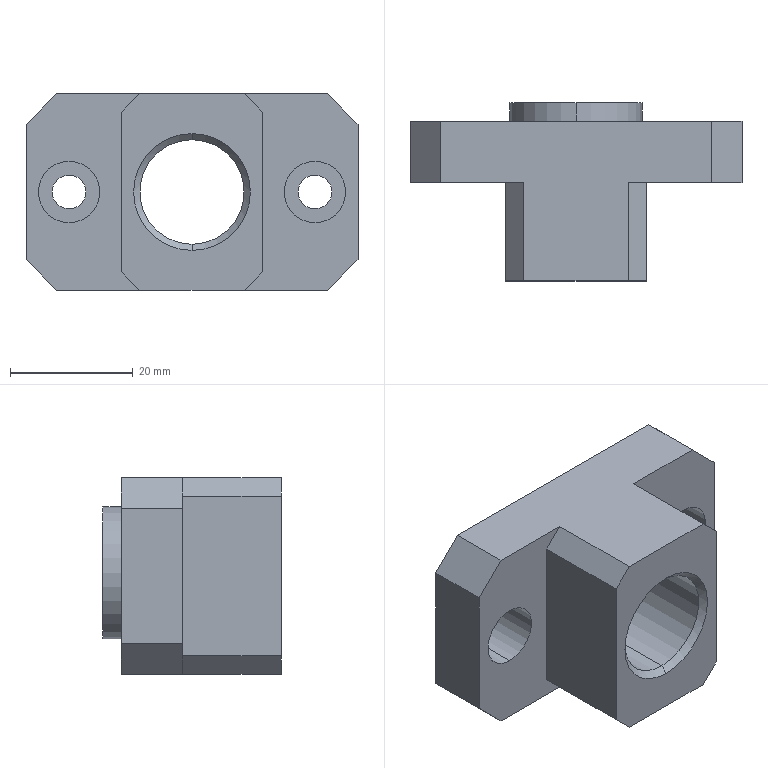Part | SolidWorks | features Chamfer 4, HoleWzd 2, Extrusion 1, ICE 1 | 1 solid | 37 faces | box 54 x 29 x 32 mm | volume 21498 mm3 | plane 21 | cylinder 12 | cone 4 | commonest cylinder face diameters 5.5 x4 10 x4 17 x2 21.5 x2
STEP:
#1=CARTESIAN_POINT('',(0.,-15.009,24.5));
#2=VERTEX_POINT('',#1);
#3=CARTESIAN_POINT('',(0.,-15.009,7.5));
#4=VERTEX_POINT('',#3);
#5=CARTESIAN_POINT('',(0.,-15.009,16.));
#6=DIRECTION('',(0.,-1.,0.));
#7=DIRECTION('',(0.,0.,1.));
#8=AXIS2_PLACEMENT_3D('',#5,#6,#7);
#9=CIRCLE('',#8,8.5);
#10=EDGE_CURVE('',#2,#4,#9,.T.);
#11=ORIENTED_EDGE('',*,*,#10,.F.);
#12=CARTESIAN_POINT('',(0.,-16.009,25.5));
#13=VERTEX_POINT('',#12);
#14=CARTESIAN_POINT('',(0.,-15.009,24.5));
#15=DIRECTION('',(0.,-0.7071,0.7071));
#16=VECTOR('',#15,1000.);
#17=LINE('',#14,#16);
#18=EDGE_CURVE('',#2,#13,#17,.T.);
#19=ORIENTED_EDGE('',*,*,#18,.T.);
#20=CARTESIAN_POINT('',(0.,-16.009,6.5));
#21=VERTEX_POINT('',#20);
#22=CARTESIAN_POINT('',(0.,-16.009,16.));
#23=DIRECTION('',(0.,1.,0.));
#24=DIRECTION('',(0.,0.,1.));
#25=AXIS2_PLACEMENT_3D('',#22,#23,#24);
#26=CIRCLE('',#25,9.5);
#27=EDGE_CURVE('',#21,#13,#26,.T.);
#28=ORIENTED_EDGE('',*,*,#27,.F.);
#29=CARTESIAN_POINT('',(0.,-15.009,7.5));
#30=DIRECTION('',(0.,-0.7071,-0.7071));
#31=VECTOR('',#30,1000.);
#32=LINE('',#29,#31);
#33=EDGE_CURVE('',#4,#21,#32,.T.);
#34=ORIENTED_EDGE('',*,*,#33,.F.);
#35=EDGE_LOOP('',(#11,#19,#28,#34));
#36=FACE_OUTER_BOUND('',#35,.T.);
#37=CARTESIAN_POINT('',(0.,-15.009,16.));
#38=DIRECTION('',(0.,-1.,0.));
#39=DIRECTION('',(0.,0.,-1.));
#40=AXIS2_PLACEMENT_3D('',#37,#38,#39);
#41=CONICAL_SURFACE('',#40,8.5,0.7854);
#42=ADVANCED_FACE('',(#36),#41,.F.);
#43=CARTESIAN_POINT('',(0.,12.491,7.5));
#44=VERTEX_POINT('',#43);
#45=CARTESIAN_POINT('',(0.,12.491,24.5));
#46=VERTEX_POINT('',#45);
#47=CARTESIAN_POINT('',(0.,12.491,16.));
#48=DIRECTION('',(0.,1.,0.));
#49=DIRECTION('',(0.,0.,1.));
#50=AXIS2_PLACEMENT_3D('',#47,#48,#49);
#51=CIRCLE('',#50,8.5);
#52=EDGE_CURVE('',#44,#46,#51,.T.);
#53=ORIENTED_EDGE('',*,*,#52,.F.);
#54=CARTESIAN_POINT('',(0.,12.991,7.));
#55=VERTEX_POINT('',#54);
#56=CARTESIAN_POINT('',(0.,12.991,7.));
#57=DIRECTION('',(0.,0.7071,-0.7071));
#58=VECTOR('',#57,1000.);
#59=LINE('',#56,#58);
#60=EDGE_CURVE('',#44,#55,#59,.T.);
#61=ORIENTED_EDGE('',*,*,#60,.T.);
#62=CARTESIAN_POINT('',(0.,12.991,25.));
#63=VERTEX_POINT('',#62);
#64=CARTESIAN_POINT('',(0.,12.991,16.));
#65=DIRECTION('',(0.,-1.,0.));
#66=DIRECTION('',(0.,0.,1.));
#67=AXIS2_PLACEMENT_3D('',#64,#65,#66);
#68=CIRCLE('',#67,9.);
#69=EDGE_CURVE('',#63,#55,#68,.T.);
#70=ORIENTED_EDGE('',*,*,#69,.F.);
#71=CARTESIAN_POINT('',(0.,12.991,25.));
#72=DIRECTION('',(0.,0.7071,0.7071));
#73=VECTOR('',#72,1000.);
#74=LINE('',#71,#73);
#75=EDGE_CURVE('',#46,#63,#74,.T.);
#76=ORIENTED_EDGE('',*,*,#75,.F.);
#77=EDGE_LOOP('',(#53,#61,#70,#76));
#78=FACE_OUTER_BOUND('',#77,.T.);
#79=CARTESIAN_POINT('',(0.,12.991,16.));
#80=DIRECTION('',(0.,1.,0.));
#81=DIRECTION('',(0.,0.,1.));
#82=AXIS2_PLACEMENT_3D('',#79,#80,#81);
#83=CONICAL_SURFACE('',#82,9.,0.7854);
#84=ADVANCED_FACE('',(#78),#83,.F.);
#85=ORIENTED_EDGE('',*,*,#52,.T.);
#86=CARTESIAN_POINT('',(0.,-16.009,24.5));
#87=DIRECTION('',(0.,-1.,0.));
#88=VECTOR('',#87,1000.);
#89=LINE('',#86,#88);
#90=EDGE_CURVE('',#46,#2,#89,.T.);
#91=ORIENTED_EDGE('',*,*,#90,.T.);
#92=ORIENTED_EDGE('',*,*,#10,.T.);
#93=CARTESIAN_POINT('',(0.,-16.009,7.5));
#94=DIRECTION('',(0.,-1.,0.));
#95=VECTOR('',#94,1000.);
#96=LINE('',#93,#95);
#97=EDGE_CURVE('',#44,#4,#96,.T.);
#98=ORIENTED_EDGE('',*,*,#97,.F.);
#99=EDGE_LOOP('',(#85,#91,#92,#98));
#100=FACE_OUTER_BOUND('',#99,.T.);
#101=CARTESIAN_POINT('',(0.,-16.009,16.));
#102=DIRECTION('',(0.,-1.,0.));
#103=DIRECTION('',(0.,0.,-1.));
#104=AXIS2_PLACEMENT_3D('',#101,#102,#103);
#105=CYLINDRICAL_SURFACE('',#104,8.5);
#106=ADVANCED_FACE('',(#100),#105,.F.);
#107=CARTESIAN_POINT('',(20.,6.991,21.));
#108=VERTEX_POINT('',#107);
#109=CARTESIAN_POINT('',(20.,6.991,11.));
#110=VERTEX_POINT('',#109);
#111=CARTESIAN_POINT('',(20.,6.991,16.));
#112=DIRECTION('',(0.,-1.,0.));
#113=DIRECTION('',(0.,0.,-1.));
#114=AXIS2_PLACEMENT_3D('',#111,#112,#113);
#115=CIRCLE('',#114,5.);
#116=EDGE_CURVE('',#108,#110,#115,.T.);
#117=ORIENTED_EDGE('',*,*,#116,.F.);
#118=CARTESIAN_POINT('',(20.,-0.00863,21.));
#119=VERTEX_POINT('',#118);
#120=CARTESIAN_POINT('',(20.,-0.00863,21.));
#121=DIRECTION('',(0.,-1.,0.));
#122=VECTOR('',#121,1000.);
#123=LINE('',#120,#122);
#124=EDGE_CURVE('',#108,#119,#123,.T.);
#125=ORIENTED_EDGE('',*,*,#124,.T.);
#126=CARTESIAN_POINT('',(20.,-0.00863,11.));
#127=VERTEX_POINT('',#126);
#128=CARTESIAN_POINT('',(20.,-0.00863,16.));
#129=DIRECTION('',(0.,-1.,0.));
#130=DIRECTION('',(0.,0.,-1.));
#131=AXIS2_PLACEMENT_3D('',#128,#129,#130);
#132=CIRCLE('',#131,5.);
#133=EDGE_CURVE('',#119,#127,#132,.T.);
#134=ORIENTED_EDGE('',*,*,#133,.T.);
#135=CARTESIAN_POINT('',(20.,-0.00863,11.));
#136=DIRECTION('',(0.,-1.,0.));
#137=VECTOR('',#136,1000.);
#138=LINE('',#135,#137);
#139=EDGE_CURVE('',#110,#127,#138,.T.);
#140=ORIENTED_EDGE('',*,*,#139,.F.);
#141=EDGE_LOOP('',(#117,#125,#134,#140));
#142=FACE_OUTER_BOUND('',#141,.T.);
#143=CARTESIAN_POINT('',(20.,-0.00863,16.));
#144=DIRECTION('',(0.,-1.,0.));
#145=DIRECTION('',(0.,0.,-1.));
#146=AXIS2_PLACEMENT_3D('',#143,#144,#145);
#147=CYLINDRICAL_SURFACE('',#146,5.);
#148=ADVANCED_FACE('',(#142),#147,.F.);
#149=CARTESIAN_POINT('',(20.,9.991,18.75));
#150=VERTEX_POINT('',#149);
#151=CARTESIAN_POINT('',(20.,9.991,13.25));
#152=VERTEX_POINT('',#151);
#153=CARTESIAN_POINT('',(20.,9.991,16.));
#154=DIRECTION('',(0.,-1.,0.));
#155=DIRECTION('',(0.,0.,-1.));
#156=AXIS2_PLACEMENT_3D('',#153,#154,#155);
#157=CIRCLE('',#156,2.75);
#158=EDGE_CURVE('',#150,#152,#157,.T.);
#159=ORIENTED_EDGE('',*,*,#158,.F.);
#160=CARTESIAN_POINT('',(20.,6.991,18.75));
#161=VERTEX_POINT('',#160);
#162=CARTESIAN_POINT('',(20.,-0.00863,18.75));
#163=DIRECTION('',(0.,-1.,0.));
#164=VECTOR('',#163,1000.);
#165=LINE('',#162,#164);
#166=EDGE_CURVE('',#150,#161,#165,.T.);
#167=ORIENTED_EDGE('',*,*,#166,.T.);
#168=CARTESIAN_POINT('',(20.,6.991,13.25));
#169=VERTEX_POINT('',#168);
#170=CARTESIAN_POINT('',(20.,6.991,16.));
#171=DIRECTION('',(0.,-1.,0.));
#172=DIRECTION('',(0.,0.,-1.));
#173=AXIS2_PLACEMENT_3D('',#170,#171,#172);
#174=CIRCLE('',#173,2.75);
#175=EDGE_CURVE('',#161,#169,#174,.T.);
#176=ORIENTED_EDGE('',*,*,#175,.T.);
#177=CARTESIAN_POINT('',(20.,-0.00863,13.25));
#178=DIRECTION('',(0.,-1.,0.));
#179=VECTOR('',#178,1000.);
#180=LINE('',#177,#179);
#181=EDGE_CURVE('',#152,#169,#180,.T.);
#182=ORIENTED_EDGE('',*,*,#181,.F.);
#183=EDGE_LOOP('',(#159,#167,#176,#182));
#184=FACE_OUTER_BOUND('',#183,.T.);
#185=CARTESIAN_POINT('',(20.,-0.00863,16.));
#186=DIRECTION('',(0.,-1.,0.));
#187=DIRECTION('',(0.,0.,-1.));
#188=AXIS2_PLACEMENT_3D('',#185,#186,#187);
#189=CYLINDRICAL_SURFACE('',#188,2.75);
#190=ADVANCED_FACE('',(#184),#189,.F.);
#191=CARTESIAN_POINT('',(-20.,6.991,21.));
#192=VERTEX_POINT('',#191);
#193=CARTESIAN_POINT('',(-20.,6.991,11.));
#194=VERTEX_POINT('',#193);
#195=CARTESIAN_POINT('',(-20.,6.991,16.));
#196=DIRECTION('',(0.,-1.,0.));
#197=DIRECTION('',(0.,0.,-1.));
#198=AXIS2_PLACEMENT_3D('',#195,#196,#197);
#199=CIRCLE('',#198,5.);
#200=EDGE_CURVE('',#192,#194,#199,.T.);
#201=ORIENTED_EDGE('',*,*,#200,.F.);
#202=CARTESIAN_POINT('',(-20.,-0.00863,21.));
#203=VERTEX_POINT('',#202);
#204=CARTESIAN_POINT('',(-20.,-0.00863,21.));
#205=DIRECTION('',(0.,-1.,0.));
#206=VECTOR('',#205,1000.);
#207=LINE('',#204,#206);
#208=EDGE_CURVE('',#192,#203,#207,.T.);
#209=ORIENTED_EDGE('',*,*,#208,.T.);
#210=CARTESIAN_POINT('',(-20.,-0.00863,11.));
#211=VERTEX_POINT('',#210);
#212=CARTESIAN_POINT('',(-20.,-0.00863,16.));
#213=DIRECTION('',(0.,-1.,0.));
#214=DIRECTION('',(0.,0.,-1.));
#215=AXIS2_PLACEMENT_3D('',#212,#213,#214);
#216=CIRCLE('',#215,5.);
#217=EDGE_CURVE('',#203,#211,#216,.T.);
#218=ORIENTED_EDGE('',*,*,#217,.T.);
#219=CARTESIAN_POINT('',(-20.,-0.00863,11.));
#220=DIRECTION('',(0.,-1.,0.));
#221=VECTOR('',#220,1000.);
#222=LINE('',#219,#221);
#223=EDGE_CURVE('',#194,#211,#222,.T.);
#224=ORIENTED_EDGE('',*,*,#223,.F.);
#225=EDGE_LOOP('',(#201,#209,#218,#224));
#226=FACE_OUTER_BOUND('',#225,.T.);
#227=CARTESIAN_POINT('',(-20.,-0.00863,16.));
#228=DIRECTION('',(0.,-1.,0.));
#229=DIRECTION('',(0.,0.,-1.));
#230=AXIS2_PLACEMENT_3D('',#227,#228,#229);
#231=CYLINDRICAL_SURFACE('',#230,5.);
#232=ADVANCED_FACE('',(#226),#231,.F.);
#233=CARTESIAN_POINT('',(-20.,9.991,18.75));
#234=VERTEX_POINT('',#233);
#235=CARTESIAN_POINT('',(-20.,9.991,13.25));
#236=VERTEX_POINT('',#235);
#237=CARTESIAN_POINT('',(-20.,9.991,16.));
#238=DIRECTION('',(0.,-1.,0.));
#239=DIRECTION('',(0.,0.,-1.));
#240=AXIS2_PLACEMENT_3D('',#237,#238,#239);
#241=CIRCLE('',#240,2.75);
#242=EDGE_CURVE('',#234,#236,#241,.T.);
#243=ORIENTED_EDGE('',*,*,#242,.F.);
#244=CARTESIAN_POINT('',(-20.,6.991,18.75));
#245=VERTEX_POINT('',#244);
#246=CARTESIAN_POINT('',(-20.,-0.00863,18.75));
#247=DIRECTION('',(0.,-1.,0.));
#248=VECTOR('',#247,1000.);
#249=LINE('',#246,#248);
#250=EDGE_CURVE('',#234,#245,#249,.T.);
#251=ORIENTED_EDGE('',*,*,#250,.T.);
#252=CARTESIAN_POINT('',(-20.,6.991,13.25));
#253=VERTEX_POINT('',#252);
#254=CARTESIAN_POINT('',(-20.,6.991,16.));
#255=DIRECTION('',(0.,-1.,0.));
#256=DIRECTION('',(0.,0.,-1.));
#257=AXIS2_PLACEMENT_3D('',#254,#255,#256);
#258=CIRCLE('',#257,2.75);
#259=EDGE_CURVE('',#245,#253,#258,.T.);
#260=ORIENTED_EDGE('',*,*,#259,.T.);
#261=CARTESIAN_POINT('',(-20.,-0.00863,13.25));
#262=DIRECTION('',(0.,-1.,0.));
#263=VECTOR('',#262,1000.);
#264=LINE('',#261,#263);
#265=EDGE_CURVE('',#236,#253,#264,.T.);
#266=ORIENTED_EDGE('',*,*,#265,.F.);
#267=EDGE_LOOP('',(#243,#251,#260,#266));
#268=FACE_OUTER_BOUND('',#267,.T.);
#269=CARTESIAN_POINT('',(-20.,-0.00863,16.));
#270=DIRECTION('',(0.,-1.,0.));
#271=DIRECTION('',(0.,0.,-1.));
#272=AXIS2_PLACEMENT_3D('',#269,#270,#271);
#273=CYLINDRICAL_SURFACE('',#272,2.75);
#274=ADVANCED_FACE('',(#268),#273,.F.);
#275=CARTESIAN_POINT('',(0.,12.991,27.297));
#276=VERTEX_POINT('',#275);
#277=CARTESIAN_POINT('',(0.,12.991,5.797));
#278=VERTEX_POINT('',#277);
#279=CARTESIAN_POINT('',(0.,12.991,16.547));
#280=DIRECTION('',(0.,1.,0.));
#281=DIRECTION('',(0.,0.,1.));
#282=AXIS2_PLACEMENT_3D('',#279,#280,#281);
#283=CIRCLE('',#282,10.75);
#284=EDGE_CURVE('',#276,#278,#283,.T.);
#285=ORIENTED_EDGE('',*,*,#284,.F.);
#286=CARTESIAN_POINT('',(0.,9.991,27.297));
#287=VERTEX_POINT('',#286);
#288=CARTESIAN_POINT('',(0.,12.991,27.297));
#289=DIRECTION('',(0.,-1.,0.));
#290=VECTOR('',#289,1000.);
#291=LINE('',#288,#290);
#292=EDGE_CURVE('',#276,#287,#291,.T.);
#293=ORIENTED_EDGE('',*,*,#292,.T.);
#294=CARTESIAN_POINT('',(0.,9.991,5.797));
#295=VERTEX_POINT('',#294);
#296=CARTESIAN_POINT('',(0.,9.991,16.547));
#297=DIRECTION('',(0.,1.,0.));
#298=DIRECTION('',(0.,0.,1.));
#299=AXIS2_PLACEMENT_3D('',#296,#297,#298);
#300=CIRCLE('',#299,10.75);
#301=EDGE_CURVE('',#287,#295,#300,.T.);
#302=ORIENTED_EDGE('',*,*,#301,.T.);
#303=CARTESIAN_POINT('',(0.,12.991,5.797));
#304=DIRECTION('',(0.,-1.,0.));
#305=VECTOR('',#304,1000.);
#306=LINE('',#303,#305);
#307=EDGE_CURVE('',#278,#295,#306,.T.);
#308=ORIENTED_EDGE('',*,*,#307,.F.);
#309=EDGE_LOOP('',(#285,#293,#302,#308));
#310=FACE_OUTER_BOUND('',#309,.T.);
#311=CARTESIAN_POINT('',(0.,12.991,16.547));
#312=DIRECTION('',(0.,-1.,0.));
#313=DIRECTION('',(0.,0.,-1.));
#314=AXIS2_PLACEMENT_3D('',#311,#312,#313);
#315=CYLINDRICAL_SURFACE('',#314,10.75);
#316=ADVANCED_FACE('',(#310),#315,.T.);
#317=CARTESIAN_POINT('',(20.,-0.00863,16.));
#318=DIRECTION('',(0.,-1.,0.));
#319=DIRECTION('',(0.,0.,-1.));
#320=AXIS2_PLACEMENT_3D('',#317,#318,#319);
#321=CIRCLE('',#320,5.);
#322=EDGE_CURVE('',#127,#119,#321,.T.);
#323=ORIENTED_EDGE('',*,*,#322,.F.);
#324=ORIENTED_EDGE('',*,*,#133,.F.);
#325=EDGE_LOOP('',(#323,#324));
#326=FACE_BOUND('',#325,.T.);
#327=CARTESIAN_POINT('',(27.,-0.00863,27.));
#328=VERTEX_POINT('',#327);
#329=CARTESIAN_POINT('',(27.,-0.00863,5.));
#330=VERTEX_POINT('',#329);
#331=CARTESIAN_POINT('',(27.,-0.00863,32.));
#332=DIRECTION('',(0.,0.,-1.));
#333=VECTOR('',#332,1000.);
#334=LINE('',#331,#333);
#335=EDGE_CURVE('',#328,#330,#334,.T.);
#336=ORIENTED_EDGE('',*,*,#335,.F.);
#337=CARTESIAN_POINT('',(22.,-0.00863,32.));
#338=VERTEX_POINT('',#337);
#339=CARTESIAN_POINT('',(22.,-0.00863,32.));
#340=DIRECTION('',(-0.7071,0.,0.7071));
#341=VECTOR('',#340,1000.);
#342=LINE('',#339,#341);
#343=EDGE_CURVE('',#328,#338,#342,.T.);
#344=ORIENTED_EDGE('',*,*,#343,.T.);
#345=CARTESIAN_POINT('',(8.5,-0.00863,32.));
#346=VERTEX_POINT('',#345);
#347=CARTESIAN_POINT('',(11.5,-0.00863,32.));
#348=DIRECTION('',(1.,0.,0.));
#349=VECTOR('',#348,1000.);
#350=LINE('',#347,#349);
#351=EDGE_CURVE('',#346,#338,#350,.T.);
#352=ORIENTED_EDGE('',*,*,#351,.F.);
#353=CARTESIAN_POINT('',(11.5,-0.00863,29.));
#354=VERTEX_POINT('',#353);
#355=CARTESIAN_POINT('',(10.,-0.00863,30.5));
#356=DIRECTION('',(0.7071,0.,-0.7071));
#357=VECTOR('',#356,1000.);
#358=LINE('',#355,#357);
#359=EDGE_CURVE('',#346,#354,#358,.T.);
#360=ORIENTED_EDGE('',*,*,#359,.T.);
#361=CARTESIAN_POINT('',(11.5,-0.00863,3.));
#362=VERTEX_POINT('',#361);
#363=CARTESIAN_POINT('',(11.5,-0.00863,32.));
#364=DIRECTION('',(0.,0.,-1.));
#365=VECTOR('',#364,1000.);
#366=LINE('',#363,#365);
#367=EDGE_CURVE('',#354,#362,#366,.T.);
#368=ORIENTED_EDGE('',*,*,#367,.T.);
#369=CARTESIAN_POINT('',(8.5,-0.00863,0.));
#370=VERTEX_POINT('',#369);
#371=CARTESIAN_POINT('',(26.,-0.00863,17.5));
#372=DIRECTION('',(-0.7071,0.,-0.7071));
#373=VECTOR('',#372,1000.);
#374=LINE('',#371,#373);
#375=EDGE_CURVE('',#362,#370,#374,.T.);
#376=ORIENTED_EDGE('',*,*,#375,.T.);
#377=CARTESIAN_POINT('',(22.,-0.00863,0.));
#378=VERTEX_POINT('',#377);
#379=CARTESIAN_POINT('',(11.5,-0.00863,0.));
#380=DIRECTION('',(1.,0.,0.));
#381=VECTOR('',#380,1000.);
#382=LINE('',#379,#381);
#383=EDGE_CURVE('',#370,#378,#382,.T.);
#384=ORIENTED_EDGE('',*,*,#383,.T.);
#385=CARTESIAN_POINT('',(27.,-0.00863,5.));
#386=DIRECTION('',(0.7071,0.,0.7071));
#387=VECTOR('',#386,1000.);
#388=LINE('',#385,#387);
#389=EDGE_CURVE('',#378,#330,#388,.T.);
#390=ORIENTED_EDGE('',*,*,#389,.T.);
#391=EDGE_LOOP('',(#336,#344,#352,#360,#368,#376,#384,#390));
#392=FACE_OUTER_BOUND('',#391,.T.);
#393=CARTESIAN_POINT('',(11.5,-0.00863,32.));
#394=DIRECTION('',(0.,1.,0.));
#395=DIRECTION('',(-1.,0.,0.));
#396=AXIS2_PLACEMENT_3D('',#393,#394,#395);
#397=PLANE('',#396);
#398=ADVANCED_FACE('',(#326,#392),#397,.F.);
#399=CARTESIAN_POINT('',(27.,9.991,27.));
#400=VERTEX_POINT('',#399);
#401=CARTESIAN_POINT('',(27.,9.991,5.));
#402=VERTEX_POINT('',#401);
#403=CARTESIAN_POINT('',(27.,9.991,32.));
#404=DIRECTION('',(0.,0.,-1.));
#405=VECTOR('',#404,1000.);
#406=LINE('',#403,#405);
#407=EDGE_CURVE('',#400,#402,#406,.T.);
#408=ORIENTED_EDGE('',*,*,#407,.F.);
#409=CARTESIAN_POINT('',(27.,-0.00863,27.));
#410=DIRECTION('',(0.,-1.,0.));
#411=VECTOR('',#410,1000.);
#412=LINE('',#409,#411);
#413=EDGE_CURVE('',#400,#328,#412,.T.);
#414=ORIENTED_EDGE('',*,*,#413,.T.);
#415=ORIENTED_EDGE('',*,*,#335,.T.);
#416=CARTESIAN_POINT('',(27.,-0.00863,5.));
#417=DIRECTION('',(0.,1.,0.));
#418=VECTOR('',#417,1000.);
#419=LINE('',#416,#418);
#420=EDGE_CURVE('',#330,#402,#419,.T.);
#421=ORIENTED_EDGE('',*,*,#420,.T.);
#422=EDGE_LOOP('',(#408,#414,#415,#421));
#423=FACE_OUTER_BOUND('',#422,.T.);
#424=CARTESIAN_POINT('',(27.,-0.00863,32.));
#425=DIRECTION('',(-1.,0.,0.));
#426=DIRECTION('',(0.,0.,1.));
#427=AXIS2_PLACEMENT_3D('',#424,#425,#426);
#428=PLANE('',#427);
#429=ADVANCED_FACE('',(#423),#428,.F.);
#430=CARTESIAN_POINT('',(20.,9.991,16.));
#431=DIRECTION('',(0.,-1.,0.));
#432=DIRECTION('',(0.,0.,-1.));
#433=AXIS2_PLACEMENT_3D('',#430,#431,#432);
#434=CIRCLE('',#433,2.75);
#435=EDGE_CURVE('',#152,#150,#434,.T.);
#436=ORIENTED_EDGE('',*,*,#435,.T.);
#437=ORIENTED_EDGE('',*,*,#158,.T.);
#438=EDGE_LOOP('',(#436,#437));
#439=FACE_BOUND('',#438,.T.);
#440=CARTESIAN_POINT('',(-20.,9.991,16.));
#441=DIRECTION('',(0.,-1.,0.));
#442=DIRECTION('',(0.,0.,-1.));
#443=AXIS2_PLACEMENT_3D('',#440,#441,#442);
#444=CIRCLE('',#443,2.75);
#445=EDGE_CURVE('',#236,#234,#444,.T.);
#446=ORIENTED_EDGE('',*,*,#445,.T.);
#447=ORIENTED_EDGE('',*,*,#242,.T.);
#448=EDGE_LOOP('',(#446,#447));
#449=FACE_BOUND('',#448,.T.);
#450=CARTESIAN_POINT('',(0.,9.991,16.547));
#451=DIRECTION('',(0.,1.,0.));
#452=DIRECTION('',(0.,0.,1.));
#453=AXIS2_PLACEMENT_3D('',#450,#451,#452);
#454=CIRCLE('',#453,10.75);
#455=EDGE_CURVE('',#295,#287,#454,.T.);
#456=ORIENTED_EDGE('',*,*,#455,.F.);
#457=ORIENTED_EDGE('',*,*,#301,.F.);
#458=EDGE_LOOP('',(#456,#457));
#459=FACE_BOUND('',#458,.T.);
#460=CARTESIAN_POINT('',(22.,9.991,32.));
#461=VERTEX_POINT('',#460);
#462=CARTESIAN_POINT('',(-22.,9.991,32.));
#463=VERTEX_POINT('',#462);
#464=CARTESIAN_POINT('',(-27.,9.991,32.));
#465=DIRECTION('',(-1.,0.,0.));
#466=VECTOR('',#465,1000.);
#467=LINE('',#464,#466);
#468=EDGE_CURVE('',#461,#463,#467,.T.);
#469=ORIENTED_EDGE('',*,*,#468,.F.);
#470=CARTESIAN_POINT('',(22.,9.991,32.));
#471=DIRECTION('',(0.7071,0.,-0.7071));
#472=VECTOR('',#471,1000.);
#473=LINE('',#470,#472);
#474=EDGE_CURVE('',#461,#400,#473,.T.);
#475=ORIENTED_EDGE('',*,*,#474,.T.);
#476=ORIENTED_EDGE('',*,*,#407,.T.);
#477=CARTESIAN_POINT('',(22.,9.991,0.));
#478=VERTEX_POINT('',#477);
#479=CARTESIAN_POINT('',(27.,9.991,5.));
#480=DIRECTION('',(-0.7071,0.,-0.7071));
#481=VECTOR('',#480,1000.);
#482=LINE('',#479,#481);
#483=EDGE_CURVE('',#402,#478,#482,.T.);
#484=ORIENTED_EDGE('',*,*,#483,.T.);
#485=CARTESIAN_POINT('',(-22.,9.991,0.));
#486=VERTEX_POINT('',#485);
#487=CARTESIAN_POINT('',(-27.,9.991,0.));
#488=DIRECTION('',(-1.,0.,0.));
#489=VECTOR('',#488,1000.);
#490=LINE('',#487,#489);
#491=EDGE_CURVE('',#478,#486,#490,.T.);
#492=ORIENTED_EDGE('',*,*,#491,.T.);
#493=CARTESIAN_POINT('',(-27.,9.991,5.));
#494=VERTEX_POINT('',#493);
#495=CARTESIAN_POINT('',(-27.,9.991,5.));
#496=DIRECTION('',(-0.7071,0.,0.7071));
#497=VECTOR('',#496,1000.);
#498=LINE('',#495,#497);
#499=EDGE_CURVE('',#486,#494,#498,.T.);
#500=ORIENTED_EDGE('',*,*,#499,.T.);
#501=CARTESIAN_POINT('',(-27.,9.991,27.));
#502=VERTEX_POINT('',#501);
#503=CARTESIAN_POINT('',(-27.,9.991,32.));
#504=DIRECTION('',(0.,0.,-1.));
#505=VECTOR('',#504,1000.);
#506=LINE('',#503,#505);
#507=EDGE_CURVE('',#502,#494,#506,.T.);
#508=ORIENTED_EDGE('',*,*,#507,.F.);
#509=CARTESIAN_POINT('',(-22.,9.991,32.));
#510=DIRECTION('',(0.7071,0.,0.7071));
#511=VECTOR('',#510,1000.);
#512=LINE('',#509,#511);
#513=EDGE_CURVE('',#502,#463,#512,.T.);
#514=ORIENTED_EDGE('',*,*,#513,.T.);
#515=EDGE_LOOP('',(#469,#475,#476,#484,#492,#500,#508,#514));
#516=FACE_OUTER_BOUND('',#515,.T.);
#517=CARTESIAN_POINT('',(-27.,9.991,32.));
#518=DIRECTION('',(0.,-1.,0.));
#519=DIRECTION('',(0.,0.,-1.));
#520=AXIS2_PLACEMENT_3D('',#517,#518,#519);
#521=PLANE('',#520);
#522=ADVANCED_FACE('',(#439,#449,#459,#516),#521,.F.);
#523=CARTESIAN_POINT('',(-27.,-0.00863,27.));
#524=VERTEX_POINT('',#523);
#525=CARTESIAN_POINT('',(-27.,-0.00863,5.));
#526=VERTEX_POINT('',#525);
#527=CARTESIAN_POINT('',(-27.,-0.00863,32.));
#528=DIRECTION('',(0.,0.,-1.));
#529=VECTOR('',#528,1000.);
#530=LINE('',#527,#529);
#531=EDGE_CURVE('',#524,#526,#530,.T.);
#532=ORIENTED_EDGE('',*,*,#531,.F.);
#533=CARTESIAN_POINT('',(-27.,9.991,27.));
#534=DIRECTION('',(0.,1.,0.));
#535=VECTOR('',#534,1000.);
#536=LINE('',#533,#535);
#537=EDGE_CURVE('',#524,#502,#536,.T.);
#538=ORIENTED_EDGE('',*,*,#537,.T.);
#539=ORIENTED_EDGE('',*,*,#507,.T.);
#540=CARTESIAN_POINT('',(-27.,-0.00863,5.));
#541=DIRECTION('',(0.,-1.,0.));
#542=VECTOR('',#541,1000.);
#543=LINE('',#540,#542);
#544=EDGE_CURVE('',#494,#526,#543,.T.);
#545=ORIENTED_EDGE('',*,*,#544,.T.);
#546=EDGE_LOOP('',(#532,#538,#539,#545));
#547=FACE_OUTER_BOUND('',#546,.T.);
#548=CARTESIAN_POINT('',(-27.,-0.00863,32.));
#549=DIRECTION('',(1.,0.,0.));
#550=DIRECTION('',(0.,0.,-1.));
#551=AXIS2_PLACEMENT_3D('',#548,#549,#550);
#552=PLANE('',#551);
#553=ADVANCED_FACE('',(#547),#552,.F.);
#554=CARTESIAN_POINT('',(-20.,-0.00863,16.));
#555=DIRECTION('',(0.,-1.,0.));
#556=DIRECTION('',(0.,0.,-1.));
#557=AXIS2_PLACEMENT_3D('',#554,#555,#556);
#558=CIRCLE('',#557,5.);
#559=EDGE_CURVE('',#211,#203,#558,.T.);
#560=ORIENTED_EDGE('',*,*,#559,.F.);
#561=ORIENTED_EDGE('',*,*,#217,.F.);
#562=EDGE_LOOP('',(#560,#561));
#563=FACE_BOUND('',#562,.T.);
#564=CARTESIAN_POINT('',(-22.,-0.00863,32.));
#565=VERTEX_POINT('',#564);
#566=CARTESIAN_POINT('',(-8.5,-0.00863,32.));
#567=VERTEX_POINT('',#566);
#568=CARTESIAN_POINT('',(-11.5,-0.00863,32.));
#569=DIRECTION('',(1.,0.,0.));
#570=VECTOR('',#569,1000.);
#571=LINE('',#568,#570);
#572=EDGE_CURVE('',#565,#567,#571,.T.);
#573=ORIENTED_EDGE('',*,*,#572,.F.);
#574=CARTESIAN_POINT('',(-22.,-0.00863,32.));
#575=DIRECTION('',(-0.7071,0.,-0.7071));
#576=VECTOR('',#575,1000.);
#577=LINE('',#574,#576);
#578=EDGE_CURVE('',#565,#524,#577,.T.);
#579=ORIENTED_EDGE('',*,*,#578,.T.);
#580=ORIENTED_EDGE('',*,*,#531,.T.);
#581=CARTESIAN_POINT('',(-22.,-0.00863,0.));
#582=VERTEX_POINT('',#581);
#583=CARTESIAN_POINT('',(-27.,-0.00863,5.));
#584=DIRECTION('',(0.7071,0.,-0.7071));
#585=VECTOR('',#584,1000.);
#586=LINE('',#583,#585);
#587=EDGE_CURVE('',#526,#582,#586,.T.);
#588=ORIENTED_EDGE('',*,*,#587,.T.);
#589=CARTESIAN_POINT('',(-8.5,-0.00863,0.));
#590=VERTEX_POINT('',#589);
#591=CARTESIAN_POINT('',(-11.5,-0.00863,0.));
#592=DIRECTION('',(1.,0.,0.));
#593=VECTOR('',#592,1000.);
#594=LINE('',#591,#593);
#595=EDGE_CURVE('',#582,#590,#594,.T.);
#596=ORIENTED_EDGE('',*,*,#595,.T.);
#597=CARTESIAN_POINT('',(-11.5,-0.00863,3.));
#598=VERTEX_POINT('',#597);
#599=CARTESIAN_POINT('',(-26.,-0.00863,17.5));
#600=DIRECTION('',(-0.7071,0.,0.7071));
#601=VECTOR('',#600,1000.);
#602=LINE('',#599,#601);
#603=EDGE_CURVE('',#590,#598,#602,.T.);
#604=ORIENTED_EDGE('',*,*,#603,.T.);
#605=CARTESIAN_POINT('',(-11.5,-0.00863,29.));
#606=VERTEX_POINT('',#605);
#607=CARTESIAN_POINT('',(-11.5,-0.00863,32.));
#608=DIRECTION('',(0.,0.,-1.));
#609=VECTOR('',#608,1000.);
#610=LINE('',#607,#609);
#611=EDGE_CURVE('',#606,#598,#610,.T.);
#612=ORIENTED_EDGE('',*,*,#611,.F.);
#613=CARTESIAN_POINT('',(-10.,-0.00863,30.5));
#614=DIRECTION('',(0.7071,0.,0.7071));
#615=VECTOR('',#614,1000.);
#616=LINE('',#613,#615);
#617=EDGE_CURVE('',#606,#567,#616,.T.);
#618=ORIENTED_EDGE('',*,*,#617,.T.);
#619=EDGE_LOOP('',(#573,#579,#580,#588,#596,#604,#612,#618));
#620=FACE_OUTER_BOUND('',#619,.T.);
#621=CARTESIAN_POINT('',(-11.5,-0.00863,32.));
#622=DIRECTION('',(0.,1.,0.));
#623=DIRECTION('',(-1.,0.,0.));
#624=AXIS2_PLACEMENT_3D('',#621,#622,#623);
#625=PLANE('',#624);
#626=ADVANCED_FACE('',(#563,#620),#625,.F.);
#627=CARTESIAN_POINT('',(-11.5,-16.009,29.));
#628=VERTEX_POINT('',#627);
#629=CARTESIAN_POINT('',(-11.5,-16.009,3.));
#630=VERTEX_POINT('',#629);
#631=CARTESIAN_POINT('',(-11.5,-16.009,32.));
#632=DIRECTION('',(0.,0.,-1.));
#633=VECTOR('',#632,1000.);
#634=LINE('',#631,#633);
#635=EDGE_CURVE('',#628,#630,#634,.T.);
#636=ORIENTED_EDGE('',*,*,#635,.F.);
#637=CARTESIAN_POINT('',(-11.5,-0.00863,29.));
#638=DIRECTION('',(0.,1.,0.));
#639=VECTOR('',#638,1000.);
#640=LINE('',#637,#639);
#641=EDGE_CURVE('',#628,#606,#640,.T.);
#642=ORIENTED_EDGE('',*,*,#641,.T.);
#643=ORIENTED_EDGE('',*,*,#611,.T.);
#644=CARTESIAN_POINT('',(-11.5,-16.009,3.));
#645=DIRECTION('',(0.,-1.,0.));
#646=VECTOR('',#645,1000.);
#647=LINE('',#644,#646);
#648=EDGE_CURVE('',#598,#630,#647,.T.);
#649=ORIENTED_EDGE('',*,*,#648,.T.);
#650=EDGE_LOOP('',(#636,#642,#643,#649));
#651=FACE_OUTER_BOUND('',#650,.T.);
#652=CARTESIAN_POINT('',(-11.5,-16.009,32.));
#653=DIRECTION('',(1.,0.,0.));
#654=DIRECTION('',(0.,1.,0.));
#655=AXIS2_PLACEMENT_3D('',#652,#653,#654);
#656=PLANE('',#655);
#657=ADVANCED_FACE('',(#651),#656,.F.);
#658=ORIENTED_EDGE('',*,*,#27,.T.);
#659=CARTESIAN_POINT('',(0.,-16.009,16.));
#660=DIRECTION('',(0.,1.,0.));
#661=DIRECTION('',(0.,0.,1.));
#662=AXIS2_PLACEMENT_3D('',#659,#660,#661);
#663=CIRCLE('',#662,9.5);
#664=EDGE_CURVE('',#13,#21,#663,.T.);
#665=ORIENTED_EDGE('',*,*,#664,.T.);
#666=EDGE_LOOP('',(#658,#665));
#667=FACE_BOUND('',#666,.T.);
#668=CARTESIAN_POINT('',(-8.5,-16.009,32.));
#669=VERTEX_POINT('',#668);
#670=CARTESIAN_POINT('',(8.5,-16.009,32.));
#671=VERTEX_POINT('',#670);
#672=CARTESIAN_POINT('',(11.5,-16.009,32.));
#673=DIRECTION('',(1.,0.,0.));
#674=VECTOR('',#673,1000.);
#675=LINE('',#672,#674);
#676=EDGE_CURVE('',#669,#671,#675,.T.);
#677=ORIENTED_EDGE('',*,*,#676,.F.);
#678=CARTESIAN_POINT('',(-8.5,-16.009,32.));
#679=DIRECTION('',(-0.7071,0.,-0.7071));
#680=VECTOR('',#679,1000.);
#681=LINE('',#678,#680);
#682=EDGE_CURVE('',#669,#628,#681,.T.);
#683=ORIENTED_EDGE('',*,*,#682,.T.);
#684=ORIENTED_EDGE('',*,*,#635,.T.);
#685=CARTESIAN_POINT('',(-8.5,-16.009,0.));
#686=VERTEX_POINT('',#685);
#687=CARTESIAN_POINT('',(-11.5,-16.009,3.));
#688=DIRECTION('',(0.7071,0.,-0.7071));
#689=VECTOR('',#688,1000.);
#690=LINE('',#687,#689);
#691=EDGE_CURVE('',#630,#686,#690,.T.);
#692=ORIENTED_EDGE('',*,*,#691,.T.);
#693=CARTESIAN_POINT('',(8.5,-16.009,0.));
#694=VERTEX_POINT('',#693);
#695=CARTESIAN_POINT('',(11.5,-16.009,0.));
#696=DIRECTION('',(1.,0.,0.));
#697=VECTOR('',#696,1000.);
#698=LINE('',#695,#697);
#699=EDGE_CURVE('',#686,#694,#698,.T.);
#700=ORIENTED_EDGE('',*,*,#699,.T.);
#701=CARTESIAN_POINT('',(11.5,-16.009,3.));
#702=VERTEX_POINT('',#701);
#703=CARTESIAN_POINT('',(11.5,-16.009,3.));
#704=DIRECTION('',(0.7071,0.,0.7071));
#705=VECTOR('',#704,1000.);
#706=LINE('',#703,#705);
#707=EDGE_CURVE('',#694,#702,#706,.T.);
#708=ORIENTED_EDGE('',*,*,#707,.T.);
#709=CARTESIAN_POINT('',(11.5,-16.009,29.));
#710=VERTEX_POINT('',#709);
#711=CARTESIAN_POINT('',(11.5,-16.009,32.));
#712=DIRECTION('',(0.,0.,-1.));
#713=VECTOR('',#712,1000.);
#714=LINE('',#711,#713);
#715=EDGE_CURVE('',#710,#702,#714,.T.);
#716=ORIENTED_EDGE('',*,*,#715,.F.);
#717=CARTESIAN_POINT('',(8.5,-16.009,32.));
#718=DIRECTION('',(-0.7071,0.,0.7071));
#719=VECTOR('',#718,1000.);
#720=LINE('',#717,#719);
#721=EDGE_CURVE('',#710,#671,#720,.T.);
#722=ORIENTED_EDGE('',*,*,#721,.T.);
#723=EDGE_LOOP('',(#677,#683,#684,#692,#700,#708,#716,#722));
#724=FACE_OUTER_BOUND('',#723,.T.);
#725=CARTESIAN_POINT('',(11.5,-16.009,32.));
#726=DIRECTION('',(0.,1.,0.));
#727=DIRECTION('',(0.,0.,1.));
#728=AXIS2_PLACEMENT_3D('',#725,#726,#727);
#729=PLANE('',#728);
#730=ADVANCED_FACE('',(#667,#724),#729,.F.);
#731=ORIENTED_EDGE('',*,*,#367,.F.);
#732=CARTESIAN_POINT('',(11.5,-16.009,29.));
#733=DIRECTION('',(0.,-1.,0.));
#734=VECTOR('',#733,1000.);
#735=LINE('',#732,#734);
#736=EDGE_CURVE('',#354,#710,#735,.T.);
#737=ORIENTED_EDGE('',*,*,#736,.T.);
#738=ORIENTED_EDGE('',*,*,#715,.T.);
#739=CARTESIAN_POINT('',(11.5,-16.009,3.));
#740=DIRECTION('',(0.,1.,0.));
#741=VECTOR('',#740,1000.);
#742=LINE('',#739,#741);
#743=EDGE_CURVE('',#702,#362,#742,.T.);
#744=ORIENTED_EDGE('',*,*,#743,.T.);
#745=EDGE_LOOP('',(#731,#737,#738,#744));
#746=FACE_OUTER_BOUND('',#745,.T.);
#747=CARTESIAN_POINT('',(11.5,-16.009,32.));
#748=DIRECTION('',(-1.,0.,0.));
#749=DIRECTION('',(0.,-1.,0.));
#750=AXIS2_PLACEMENT_3D('',#747,#748,#749);
#751=PLANE('',#750);
#752=ADVANCED_FACE('',(#746),#751,.F.);
#753=ORIENTED_EDGE('',*,*,#572,.T.);
#754=CARTESIAN_POINT('',(-8.5,-16.009,32.));
#755=DIRECTION('',(0.,-1.,0.));
#756=VECTOR('',#755,1000.);
#757=LINE('',#754,#756);
#758=EDGE_CURVE('',#567,#669,#757,.T.);
#759=ORIENTED_EDGE('',*,*,#758,.T.);
#760=ORIENTED_EDGE('',*,*,#676,.T.);
#761=CARTESIAN_POINT('',(8.5,-0.00863,32.));
#762=DIRECTION('',(0.,1.,0.));
#763=VECTOR('',#762,1000.);
#764=LINE('',#761,#763);
#765=EDGE_CURVE('',#671,#346,#764,.T.);
#766=ORIENTED_EDGE('',*,*,#765,.T.);
#767=ORIENTED_EDGE('',*,*,#351,.T.);
#768=CARTESIAN_POINT('',(22.,9.991,32.));
#769=DIRECTION('',(0.,1.,0.));
#770=VECTOR('',#769,1000.);
#771=LINE('',#768,#770);
#772=EDGE_CURVE('',#338,#461,#771,.T.);
#773=ORIENTED_EDGE('',*,*,#772,.T.);
#774=ORIENTED_EDGE('',*,*,#468,.T.);
#775=CARTESIAN_POINT('',(-22.,-0.00863,32.));
#776=DIRECTION('',(0.,-1.,0.));
#777=VECTOR('',#776,1000.);
#778=LINE('',#775,#777);
#779=EDGE_CURVE('',#463,#565,#778,.T.);
#780=ORIENTED_EDGE('',*,*,#779,.T.);
#781=EDGE_LOOP('',(#753,#759,#760,#766,#767,#773,#774,#780));
#782=FACE_OUTER_BOUND('',#781,.T.);
#783=CARTESIAN_POINT('',(0.,0.,32.));
#784=DIRECTION('',(0.,0.,1.));
#785=DIRECTION('',(1.,0.,0.));
#786=AXIS2_PLACEMENT_3D('',#783,#784,#785);
#787=PLANE('',#786);
#788=ADVANCED_FACE('',(#782),#787,.T.);
#789=ORIENTED_EDGE('',*,*,#699,.F.);
#790=CARTESIAN_POINT('',(-8.5,0.,0.));
#791=DIRECTION('',(0.,1.,0.));
#792=VECTOR('',#791,1000.);
#793=LINE('',#790,#792);
#794=EDGE_CURVE('',#686,#590,#793,.T.);
#795=ORIENTED_EDGE('',*,*,#794,.T.);
#796=ORIENTED_EDGE('',*,*,#595,.F.);
#797=CARTESIAN_POINT('',(-22.,0.,0.));
#798=DIRECTION('',(0.,1.,0.));
#799=VECTOR('',#798,1000.);
#800=LINE('',#797,#799);
#801=EDGE_CURVE('',#582,#486,#800,.T.);
#802=ORIENTED_EDGE('',*,*,#801,.T.);
#803=ORIENTED_EDGE('',*,*,#491,.F.);
#804=CARTESIAN_POINT('',(22.,0.,0.));
#805=DIRECTION('',(0.,-1.,0.));
#806=VECTOR('',#805,1000.);
#807=LINE('',#804,#806);
#808=EDGE_CURVE('',#478,#378,#807,.T.);
#809=ORIENTED_EDGE('',*,*,#808,.T.);
#810=ORIENTED_EDGE('',*,*,#383,.F.);
#811=CARTESIAN_POINT('',(8.5,0.,0.));
#812=DIRECTION('',(0.,-1.,0.));
#813=VECTOR('',#812,1000.);
#814=LINE('',#811,#813);
#815=EDGE_CURVE('',#370,#694,#814,.T.);
#816=ORIENTED_EDGE('',*,*,#815,.T.);
#817=EDGE_LOOP('',(#789,#795,#796,#802,#803,#809,#810,#816));
#818=FACE_OUTER_BOUND('',#817,.T.);
#819=CARTESIAN_POINT('',(0.,0.,0.));
#820=DIRECTION('',(0.,0.,1.));
#821=DIRECTION('',(1.,0.,0.));
#822=AXIS2_PLACEMENT_3D('',#819,#820,#821);
#823=PLANE('',#822);
#824=ADVANCED_FACE('',(#818),#823,.F.);
#825=ORIENTED_EDGE('',*,*,#343,.F.);
#826=ORIENTED_EDGE('',*,*,#413,.F.);
#827=ORIENTED_EDGE('',*,*,#474,.F.);
#828=ORIENTED_EDGE('',*,*,#772,.F.);
#829=EDGE_LOOP('',(#825,#826,#827,#828));
#830=FACE_OUTER_BOUND('',#829,.T.);
#831=CARTESIAN_POINT('',(22.,0.,32.));
#832=DIRECTION('',(0.7071,0.,0.7071));
#833=DIRECTION('',(0.,-1.,0.));
#834=AXIS2_PLACEMENT_3D('',#831,#832,#833);
#835=PLANE('',#834);
#836=ADVANCED_FACE('',(#830),#835,.T.);
#837=ORIENTED_EDGE('',*,*,#389,.F.);
#838=ORIENTED_EDGE('',*,*,#808,.F.);
#839=ORIENTED_EDGE('',*,*,#483,.F.);
#840=ORIENTED_EDGE('',*,*,#420,.F.);
#841=EDGE_LOOP('',(#837,#838,#839,#840));
#842=FACE_OUTER_BOUND('',#841,.T.);
#843=CARTESIAN_POINT('',(27.,-0.00863,5.));
#844=DIRECTION('',(-0.7071,0.,0.7071));
#845=DIRECTION('',(0.,1.,0.));
#846=AXIS2_PLACEMENT_3D('',#843,#844,#845);
#847=PLANE('',#846);
#848=ADVANCED_FACE('',(#842),#847,.F.);
#849=ORIENTED_EDGE('',*,*,#513,.F.);
#850=ORIENTED_EDGE('',*,*,#537,.F.);
#851=ORIENTED_EDGE('',*,*,#578,.F.);
#852=ORIENTED_EDGE('',*,*,#779,.F.);
#853=EDGE_LOOP('',(#849,#850,#851,#852));
#854=FACE_OUTER_BOUND('',#853,.T.);
#855=CARTESIAN_POINT('',(-22.,0.,32.));
#856=DIRECTION('',(-0.7071,0.,0.7071));
#857=DIRECTION('',(0.,1.,0.));
#858=AXIS2_PLACEMENT_3D('',#855,#856,#857);
#859=PLANE('',#858);
#860=ADVANCED_FACE('',(#854),#859,.T.);
#861=ORIENTED_EDGE('',*,*,#499,.F.);
#862=ORIENTED_EDGE('',*,*,#801,.F.);
#863=ORIENTED_EDGE('',*,*,#587,.F.);
#864=ORIENTED_EDGE('',*,*,#544,.F.);
#865=EDGE_LOOP('',(#861,#862,#863,#864));
#866=FACE_OUTER_BOUND('',#865,.T.);
#867=CARTESIAN_POINT('',(-27.,-0.00863,5.));
#868=DIRECTION('',(0.7071,0.,0.7071));
#869=DIRECTION('',(0.,-1.,0.));
#870=AXIS2_PLACEMENT_3D('',#867,#868,#869);
#871=PLANE('',#870);
#872=ADVANCED_FACE('',(#866),#871,.F.);
#873=ORIENTED_EDGE('',*,*,#292,.F.);
#874=CARTESIAN_POINT('',(0.,12.991,16.547));
#875=DIRECTION('',(0.,1.,0.));
#876=DIRECTION('',(0.,0.,1.));
#877=AXIS2_PLACEMENT_3D('',#874,#875,#876);
#878=CIRCLE('',#877,10.75);
#879=EDGE_CURVE('',#278,#276,#878,.T.);
#880=ORIENTED_EDGE('',*,*,#879,.F.);
#881=ORIENTED_EDGE('',*,*,#307,.T.);
#882=ORIENTED_EDGE('',*,*,#455,.T.);
#883=EDGE_LOOP('',(#873,#880,#881,#882));
#884=FACE_OUTER_BOUND('',#883,.T.);
#885=CARTESIAN_POINT('',(0.,12.991,16.547));
#886=DIRECTION('',(0.,-1.,0.));
#887=DIRECTION('',(0.,0.,-1.));
#888=AXIS2_PLACEMENT_3D('',#885,#886,#887);
#889=CYLINDRICAL_SURFACE('',#888,10.75);
#890=ADVANCED_FACE('',(#884),#889,.T.);
#891=ORIENTED_EDGE('',*,*,#69,.T.);
#892=CARTESIAN_POINT('',(0.,12.991,16.));
#893=DIRECTION('',(0.,-1.,0.));
#894=DIRECTION('',(0.,0.,1.));
#895=AXIS2_PLACEMENT_3D('',#892,#893,#894);
#896=CIRCLE('',#895,9.);
#897=EDGE_CURVE('',#55,#63,#896,.T.);
#898=ORIENTED_EDGE('',*,*,#897,.T.);
#899=EDGE_LOOP('',(#891,#898));
#900=FACE_BOUND('',#899,.T.);
#901=ORIENTED_EDGE('',*,*,#879,.T.);
#902=ORIENTED_EDGE('',*,*,#284,.T.);
#903=EDGE_LOOP('',(#901,#902));
#904=FACE_OUTER_BOUND('',#903,.T.);
#905=CARTESIAN_POINT('',(0.,12.991,16.547));
#906=DIRECTION('',(0.,1.,0.));
#907=DIRECTION('',(0.,0.,1.));
#908=AXIS2_PLACEMENT_3D('',#905,#906,#907);
#909=PLANE('',#908);
#910=ADVANCED_FACE('',(#900,#904),#909,.T.);
#911=ORIENTED_EDGE('',*,*,#250,.F.);
#912=ORIENTED_EDGE('',*,*,#445,.F.);
#913=ORIENTED_EDGE('',*,*,#265,.T.);
#914=CARTESIAN_POINT('',(-20.,6.991,16.));
#915=DIRECTION('',(0.,-1.,0.));
#916=DIRECTION('',(0.,0.,-1.));
#917=AXIS2_PLACEMENT_3D('',#914,#915,#916);
#918=CIRCLE('',#917,2.75);
#919=EDGE_CURVE('',#253,#245,#918,.T.);
#920=ORIENTED_EDGE('',*,*,#919,.T.);
#921=EDGE_LOOP('',(#911,#912,#913,#920));
#922=FACE_OUTER_BOUND('',#921,.T.);
#923=CARTESIAN_POINT('',(-20.,-0.00863,16.));
#924=DIRECTION('',(0.,-1.,0.));
#925=DIRECTION('',(0.,0.,-1.));
#926=AXIS2_PLACEMENT_3D('',#923,#924,#925);
#927=CYLINDRICAL_SURFACE('',#926,2.75);
#928=ADVANCED_FACE('',(#922),#927,.F.);
#929=ORIENTED_EDGE('',*,*,#919,.F.);
#930=ORIENTED_EDGE('',*,*,#259,.F.);
#931=EDGE_LOOP('',(#929,#930));
#932=FACE_BOUND('',#931,.T.);
#933=CARTESIAN_POINT('',(-20.,6.991,16.));
#934=DIRECTION('',(0.,-1.,0.));
#935=DIRECTION('',(0.,0.,-1.));
#936=AXIS2_PLACEMENT_3D('',#933,#934,#935);
#937=CIRCLE('',#936,5.);
#938=EDGE_CURVE('',#194,#192,#937,.T.);
#939=ORIENTED_EDGE('',*,*,#938,.T.);
#940=ORIENTED_EDGE('',*,*,#200,.T.);
#941=EDGE_LOOP('',(#939,#940));
#942=FACE_OUTER_BOUND('',#941,.T.);
#943=CARTESIAN_POINT('',(-17.25,6.991,16.));
#944=DIRECTION('',(0.,1.,0.));
#945=DIRECTION('',(0.,0.,1.));
#946=AXIS2_PLACEMENT_3D('',#943,#944,#945);
#947=PLANE('',#946);
#948=ADVANCED_FACE('',(#932,#942),#947,.F.);
#949=ORIENTED_EDGE('',*,*,#208,.F.);
#950=ORIENTED_EDGE('',*,*,#938,.F.);
#951=ORIENTED_EDGE('',*,*,#223,.T.);
#952=ORIENTED_EDGE('',*,*,#559,.T.);
#953=EDGE_LOOP('',(#949,#950,#951,#952));
#954=FACE_OUTER_BOUND('',#953,.T.);
#955=CARTESIAN_POINT('',(-20.,-0.00863,16.));
#956=DIRECTION('',(0.,-1.,0.));
#957=DIRECTION('',(0.,0.,-1.));
#958=AXIS2_PLACEMENT_3D('',#955,#956,#957);
#959=CYLINDRICAL_SURFACE('',#958,5.);
#960=ADVANCED_FACE('',(#954),#959,.F.);
#961=ORIENTED_EDGE('',*,*,#166,.F.);
#962=ORIENTED_EDGE('',*,*,#435,.F.);
#963=ORIENTED_EDGE('',*,*,#181,.T.);
#964=CARTESIAN_POINT('',(20.,6.991,16.));
#965=DIRECTION('',(0.,-1.,0.));
#966=DIRECTION('',(0.,0.,-1.));
#967=AXIS2_PLACEMENT_3D('',#964,#965,#966);
#968=CIRCLE('',#967,2.75);
#969=EDGE_CURVE('',#169,#161,#968,.T.);
#970=ORIENTED_EDGE('',*,*,#969,.T.);
#971=EDGE_LOOP('',(#961,#962,#963,#970));
#972=FACE_OUTER_BOUND('',#971,.T.);
#973=CARTESIAN_POINT('',(20.,-0.00863,16.));
#974=DIRECTION('',(0.,-1.,0.));
#975=DIRECTION('',(0.,0.,-1.));
#976=AXIS2_PLACEMENT_3D('',#973,#974,#975);
#977=CYLINDRICAL_SURFACE('',#976,2.75);
#978=ADVANCED_FACE('',(#972),#977,.F.);
#979=ORIENTED_EDGE('',*,*,#969,.F.);
#980=ORIENTED_EDGE('',*,*,#175,.F.);
#981=EDGE_LOOP('',(#979,#980));
#982=FACE_BOUND('',#981,.T.);
#983=CARTESIAN_POINT('',(20.,6.991,16.));
#984=DIRECTION('',(0.,-1.,0.));
#985=DIRECTION('',(0.,0.,-1.));
#986=AXIS2_PLACEMENT_3D('',#983,#984,#985);
#987=CIRCLE('',#986,5.);
#988=EDGE_CURVE('',#110,#108,#987,.T.);
#989=ORIENTED_EDGE('',*,*,#988,.T.);
#990=ORIENTED_EDGE('',*,*,#116,.T.);
#991=EDGE_LOOP('',(#989,#990));
#992=FACE_OUTER_BOUND('',#991,.T.);
#993=CARTESIAN_POINT('',(22.75,6.991,16.));
#994=DIRECTION('',(0.,1.,0.));
#995=DIRECTION('',(0.,0.,1.));
#996=AXIS2_PLACEMENT_3D('',#993,#994,#995);
#997=PLANE('',#996);
#998=ADVANCED_FACE('',(#982,#992),#997,.F.);
#999=ORIENTED_EDGE('',*,*,#124,.F.);
#1000=ORIENTED_EDGE('',*,*,#988,.F.);
#1001=ORIENTED_EDGE('',*,*,#139,.T.);
#1002=ORIENTED_EDGE('',*,*,#322,.T.);
#1003=EDGE_LOOP('',(#999,#1000,#1001,#1002));
#1004=FACE_OUTER_BOUND('',#1003,.T.);
#1005=CARTESIAN_POINT('',(20.,-0.00863,16.));
#1006=DIRECTION('',(0.,-1.,0.));
#1007=DIRECTION('',(0.,0.,-1.));
#1008=AXIS2_PLACEMENT_3D('',#1005,#1006,#1007);
#1009=CYLINDRICAL_SURFACE('',#1008,5.);
#1010=ADVANCED_FACE('',(#1004),#1009,.F.);
#1011=ORIENTED_EDGE('',*,*,#617,.F.);
#1012=ORIENTED_EDGE('',*,*,#641,.F.);
#1013=ORIENTED_EDGE('',*,*,#682,.F.);
#1014=ORIENTED_EDGE('',*,*,#758,.F.);
#1015=EDGE_LOOP('',(#1011,#1012,#1013,#1014));
#1016=FACE_OUTER_BOUND('',#1015,.T.);
#1017=CARTESIAN_POINT('',(-8.5,0.,32.));
#1018=DIRECTION('',(-0.7071,0.,0.7071));
#1019=DIRECTION('',(0.,1.,0.));
#1020=AXIS2_PLACEMENT_3D('',#1017,#1018,#1019);
#1021=PLANE('',#1020);
#1022=ADVANCED_FACE('',(#1016),#1021,.T.);
#1023=ORIENTED_EDGE('',*,*,#603,.F.);
#1024=ORIENTED_EDGE('',*,*,#794,.F.);
#1025=ORIENTED_EDGE('',*,*,#691,.F.);
#1026=ORIENTED_EDGE('',*,*,#648,.F.);
#1027=EDGE_LOOP('',(#1023,#1024,#1025,#1026));
#1028=FACE_OUTER_BOUND('',#1027,.T.);
#1029=CARTESIAN_POINT('',(-11.5,-16.009,3.));
#1030=DIRECTION('',(0.7071,0.,0.7071));
#1031=DIRECTION('',(0.,-1.,0.));
#1032=AXIS2_PLACEMENT_3D('',#1029,#1030,#1031);
#1033=PLANE('',#1032);
#1034=ADVANCED_FACE('',(#1028),#1033,.F.);
#1035=ORIENTED_EDGE('',*,*,#721,.F.);
#1036=ORIENTED_EDGE('',*,*,#736,.F.);
#1037=ORIENTED_EDGE('',*,*,#359,.F.);
#1038=ORIENTED_EDGE('',*,*,#765,.F.);
#1039=EDGE_LOOP('',(#1035,#1036,#1037,#1038));
#1040=FACE_OUTER_BOUND('',#1039,.T.);
#1041=CARTESIAN_POINT('',(8.5,0.,32.));
#1042=DIRECTION('',(0.7071,0.,0.7071));
#1043=DIRECTION('',(0.,-1.,0.));
#1044=AXIS2_PLACEMENT_3D('',#1041,#1042,#1043);
#1045=PLANE('',#1044);
#1046=ADVANCED_FACE('',(#1040),#1045,.T.);
#1047=ORIENTED_EDGE('',*,*,#707,.F.);
#1048=ORIENTED_EDGE('',*,*,#815,.F.);
#1049=ORIENTED_EDGE('',*,*,#375,.F.);
#1050=ORIENTED_EDGE('',*,*,#743,.F.);
#1051=EDGE_LOOP('',(#1047,#1048,#1049,#1050));
#1052=FACE_OUTER_BOUND('',#1051,.T.);
#1053=CARTESIAN_POINT('',(11.5,-16.009,3.));
#1054=DIRECTION('',(-0.7071,0.,0.7071));
#1055=DIRECTION('',(0.,1.,0.));
#1056=AXIS2_PLACEMENT_3D('',#1053,#1054,#1055);
#1057=PLANE('',#1056);
#1058=ADVANCED_FACE('',(#1052),#1057,.F.);
#1059=ORIENTED_EDGE('',*,*,#90,.F.);
#1060=CARTESIAN_POINT('',(0.,12.491,16.));
#1061=DIRECTION('',(0.,1.,0.));
#1062=DIRECTION('',(0.,0.,1.));
#1063=AXIS2_PLACEMENT_3D('',#1060,#1061,#1062);
#1064=CIRCLE('',#1063,8.5);
#1065=EDGE_CURVE('',#46,#44,#1064,.T.);
#1066=ORIENTED_EDGE('',*,*,#1065,.T.);
#1067=ORIENTED_EDGE('',*,*,#97,.T.);
#1068=CARTESIAN_POINT('',(0.,-15.009,16.));
#1069=DIRECTION('',(0.,-1.,0.));
#1070=DIRECTION('',(0.,0.,1.));
#1071=AXIS2_PLACEMENT_3D('',#1068,#1069,#1070);
#1072=CIRCLE('',#1071,8.5);
#1073=EDGE_CURVE('',#4,#2,#1072,.T.);
#1074=ORIENTED_EDGE('',*,*,#1073,.T.);
#1075=EDGE_LOOP('',(#1059,#1066,#1067,#1074));
#1076=FACE_OUTER_BOUND('',#1075,.T.);
#1077=CARTESIAN_POINT('',(0.,-16.009,16.));
#1078=DIRECTION('',(0.,-1.,0.));
#1079=DIRECTION('',(0.,0.,-1.));
#1080=AXIS2_PLACEMENT_3D('',#1077,#1078,#1079);
#1081=CYLINDRICAL_SURFACE('',#1080,8.5);
#1082=ADVANCED_FACE('',(#1076),#1081,.F.);
#1083=ORIENTED_EDGE('',*,*,#60,.F.);
#1084=ORIENTED_EDGE('',*,*,#1065,.F.);
#1085=ORIENTED_EDGE('',*,*,#75,.T.);
#1086=ORIENTED_EDGE('',*,*,#897,.F.);
#1087=EDGE_LOOP('',(#1083,#1084,#1085,#1086));
#1088=FACE_OUTER_BOUND('',#1087,.T.);
#1089=CARTESIAN_POINT('',(0.,12.991,16.));
#1090=DIRECTION('',(0.,1.,0.));
#1091=DIRECTION('',(0.,0.,1.));
#1092=AXIS2_PLACEMENT_3D('',#1089,#1090,#1091);
#1093=CONICAL_SURFACE('',#1092,9.,0.7854);
#1094=ADVANCED_FACE('',(#1088),#1093,.F.);
#1095=ORIENTED_EDGE('',*,*,#18,.F.);
#1096=ORIENTED_EDGE('',*,*,#1073,.F.);
#1097=ORIENTED_EDGE('',*,*,#33,.T.);
#1098=ORIENTED_EDGE('',*,*,#664,.F.);
#1099=EDGE_LOOP('',(#1095,#1096,#1097,#1098));
#1100=FACE_OUTER_BOUND('',#1099,.T.);
#1101=CARTESIAN_POINT('',(0.,-15.009,16.));
#1102=DIRECTION('',(0.,-1.,0.));
#1103=DIRECTION('',(0.,0.,-1.));
#1104=AXIS2_PLACEMENT_3D('',#1101,#1102,#1103);
#1105=CONICAL_SURFACE('',#1104,8.5,0.7854);
#1106=ADVANCED_FACE('',(#1100),#1105,.F.);
#1107=CLOSED_SHELL('',(#42,#84,#106,#148,#190,#232,#274,#316,#398,#429,#522,#553,#626,#657,#730,#752,#788,#824,#836,#848,#860,#872,#890,#910,#928,#948,#960,#978,#998,#1010,#1022,#1034,#1046,#1058,#1082,#1094,#1106));
#1108=MANIFOLD_SOLID_BREP('',#1107);
#1109=CARTESIAN_POINT('',(0.,0.,0.));
#1110=DIRECTION('',(0.,0.,1.));
#1111=DIRECTION('',(1.,0.,0.));
#1112=AXIS2_PLACEMENT_3D('',#1109,#1110,#1111);
#1113=(LENGTH_UNIT()NAMED_UNIT(*)SI_UNIT(.MILLI.,.METRE.));
#1114=UNCERTAINTY_MEASURE_WITH_UNIT(LENGTH_MEASURE(0.00001),#1113,'','');
#1115=(NAMED_UNIT(*)PLANE_ANGLE_UNIT()SI_UNIT($,.RADIAN.));
#1116=(NAMED_UNIT(*)SI_UNIT($,.STERADIAN.)SOLID_ANGLE_UNIT());
#1117=(GEOMETRIC_REPRESENTATION_CONTEXT(3)GLOBAL_UNCERTAINTY_ASSIGNED_CONTEXT((#1114))GLOBAL_UNIT_ASSIGNED_CONTEXT((#1113,#1115,#1116))REPRESENTATION_CONTEXT('',''));
#1118=ADVANCED_BREP_SHAPE_REPRESENTATION('',(#1108,#1112),#1117);